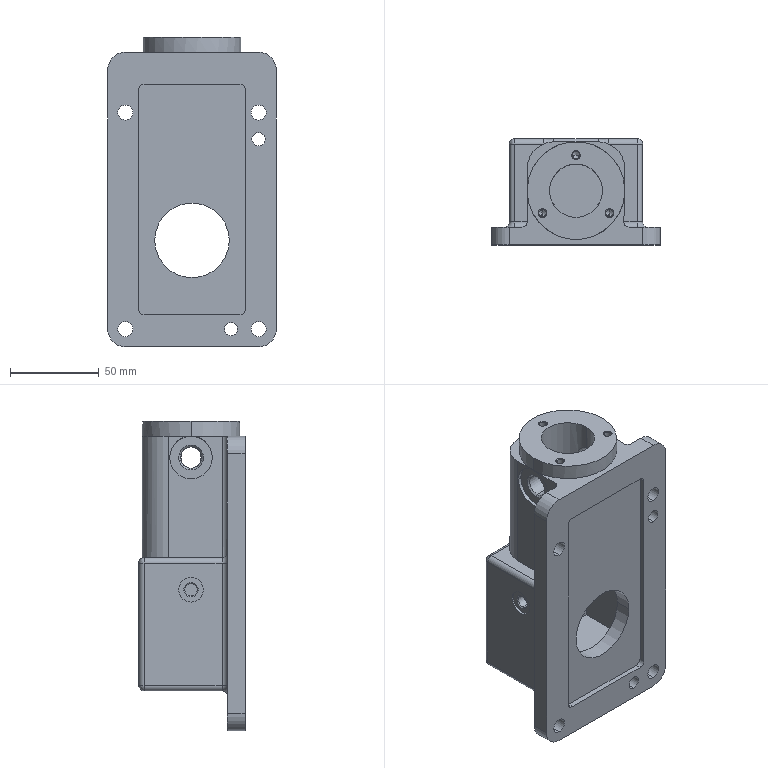Part | SolidWorks | features ICE 17, Fillet 4, HoleWzd 4, CirPattern 1, Extrusion 1, MirrorPattern 1 | 1 solid | 181 faces | box 95 x 59.897 x 174.5 mm | volume 358133 mm3 | cylinder 89 | cone 44 | plane 38 | sphere 4 | torus 4 | spline 2 | commonest cylinder face diameters 6 x22 5 x12 8.5 x8 13 x8 4.2 x6 12 x4